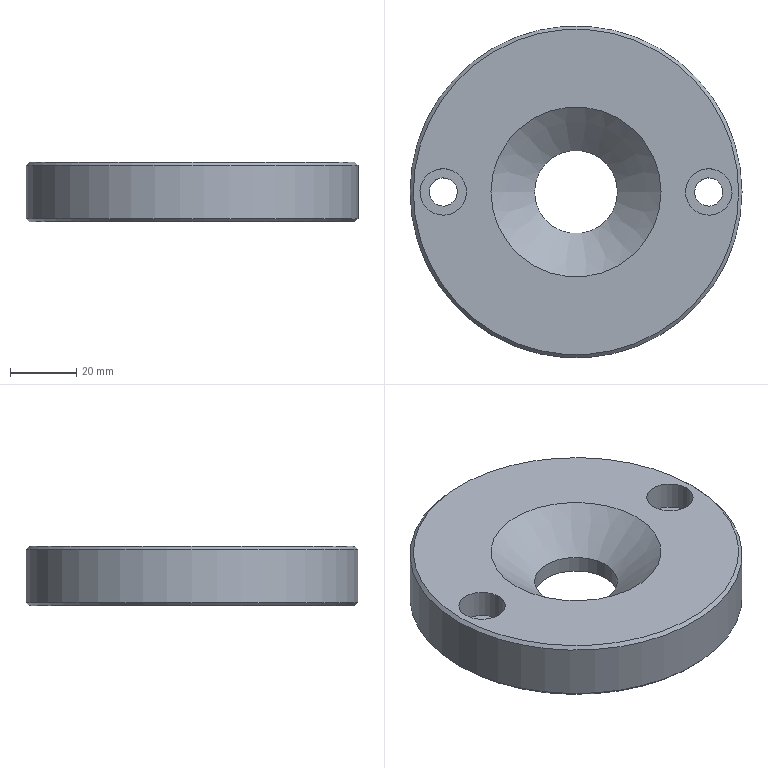Part | STEP file | P011002NF01-000 | 1 solid | 15 faces | box 100 x 100 x 18 mm | volume 119839 mm3 | cylinder 7 | plane 5 | cone 3 | commonest cylinder face diameters 8.5 x2 14 x2 25 x1 36 x1 100 x1
STEP:
#1=CARTESIAN_POINT('',(0.,0.,0.));
#2=DIRECTION('',(0.,0.,1.));
#3=DIRECTION('',(1.,0.,0.));
#4=AXIS2_PLACEMENT_3D('',#1,#2,#3);
#5=CARTESIAN_POINT('',(-12.5,0.,330.));
#6=VERTEX_POINT('',#5);
#7=CARTESIAN_POINT('',(12.5,0.,330.));
#8=VERTEX_POINT('',#7);
#9=CARTESIAN_POINT('',(0.,0.,330.));
#10=DIRECTION('',(0.,0.,1.));
#11=DIRECTION('',(-1.,0.,0.));
#12=AXIS2_PLACEMENT_3D('',#9,#10,#11);
#13=CIRCLE('',#12,12.5);
#14=CARTESIAN_POINT('',(0.,0.,330.));
#15=DIRECTION('',(0.,0.,-1.));
#16=DIRECTION('',(-0.9819,-0.1894,0.));
#17=AXIS2_PLACEMENT_3D('',#14,#15,#16);
#18=PLANE('',#17);
#19=CARTESIAN_POINT('',(12.274,2.368));
#20=CARTESIAN_POINT('',(16.375,-18.891));
#21=CARTESIAN_POINT('',(-4.086,-11.813));
#22=CARTESIAN_POINT('',(-24.547,-4.735));
#23=CARTESIAN_POINT('',(-8.187,9.446));
#24=CARTESIAN_POINT('',(8.173,23.626));
#25=CARTESIAN_POINT('',(12.274,2.368));
#26=(BOUNDED_CURVE()B_SPLINE_CURVE(2,(#19,#20,#21,#22,#23,#24,#25),.UNSPECIFIED.,.T.,.F.)B_SPLINE_CURVE_WITH_KNOTS((1,2,2,2,2,1),(-2.094,0.,2.094,4.189,6.283,8.378),.UNSPECIFIED.)CURVE()GEOMETRIC_REPRESENTATION_ITEM()RATIONAL_B_SPLINE_CURVE((1.,0.5,1.,0.5,1.,0.5,1.))REPRESENTATION_ITEM(''));
#27=(GEOMETRIC_REPRESENTATION_CONTEXT(2)PARAMETRIC_REPRESENTATION_CONTEXT()REPRESENTATION_CONTEXT('',''));
#28=DEFINITIONAL_REPRESENTATION('',(#26),#27);
#29=PCURVE('',#18,#28);
#30=CARTESIAN_POINT('',(0.,0.,289.));
#31=DIRECTION('',(0.,0.,1.));
#32=DIRECTION('',(0.9819,0.1894,0.));
#33=AXIS2_PLACEMENT_3D('',#30,#31,#32);
#34=CYLINDRICAL_SURFACE('',#33,12.5);
#35=CARTESIAN_POINT('',(9.234,41.));
#36=DIRECTION('',(1.,0.));
#37=VECTOR('',#36,1.);
#38=LINE('',#35,#37);
#39=(GEOMETRIC_REPRESENTATION_CONTEXT(2)PARAMETRIC_REPRESENTATION_CONTEXT()REPRESENTATION_CONTEXT('',''));
#40=DEFINITIONAL_REPRESENTATION('',(#38),#39);
#41=PCURVE('',#34,#40);
#42=SURFACE_CURVE('',#13,(#29,#41),.PCURVE_S1.);
#43=EDGE_CURVE('',#6,#8,#42,.T.);
#44=ORIENTED_EDGE('',*,*,#43,.T.);
#45=CARTESIAN_POINT('',(0.,0.,330.));
#46=DIRECTION('',(0.,0.,1.));
#47=DIRECTION('',(-1.,0.,0.));
#48=AXIS2_PLACEMENT_3D('',#45,#46,#47);
#49=CIRCLE('',#48,12.5);
#50=CARTESIAN_POINT('',(12.274,2.368));
#51=CARTESIAN_POINT('',(16.375,-18.891));
#52=CARTESIAN_POINT('',(-4.086,-11.813));
#53=CARTESIAN_POINT('',(-24.547,-4.735));
#54=CARTESIAN_POINT('',(-8.187,9.446));
#55=CARTESIAN_POINT('',(8.173,23.626));
#56=CARTESIAN_POINT('',(12.274,2.368));
#57=(BOUNDED_CURVE()B_SPLINE_CURVE(2,(#50,#51,#52,#53,#54,#55,#56),.UNSPECIFIED.,.T.,.F.)B_SPLINE_CURVE_WITH_KNOTS((1,2,2,2,2,1),(-2.094,0.,2.094,4.189,6.283,8.378),.UNSPECIFIED.)CURVE()GEOMETRIC_REPRESENTATION_ITEM()RATIONAL_B_SPLINE_CURVE((1.,0.5,1.,0.5,1.,0.5,1.))REPRESENTATION_ITEM(''));
#58=(GEOMETRIC_REPRESENTATION_CONTEXT(2)PARAMETRIC_REPRESENTATION_CONTEXT()REPRESENTATION_CONTEXT('',''));
#59=DEFINITIONAL_REPRESENTATION('',(#57),#58);
#60=PCURVE('',#18,#59);
#61=CARTESIAN_POINT('',(2.951,41.));
#62=DIRECTION('',(1.,0.));
#63=VECTOR('',#62,1.);
#64=LINE('',#61,#63);
#65=(GEOMETRIC_REPRESENTATION_CONTEXT(2)PARAMETRIC_REPRESENTATION_CONTEXT()REPRESENTATION_CONTEXT('',''));
#66=DEFINITIONAL_REPRESENTATION('',(#64),#65);
#67=PCURVE('',#34,#66);
#68=SURFACE_CURVE('',#49,(#60,#67),.PCURVE_S1.);
#69=EDGE_CURVE('',#8,#6,#68,.T.);
#70=ORIENTED_EDGE('',*,*,#69,.T.);
#71=EDGE_LOOP('',(#44,#70));
#72=FACE_BOUND('',#71,.T.);
#73=CARTESIAN_POINT('',(-18.,0.,330.));
#74=VERTEX_POINT('',#73);
#75=CARTESIAN_POINT('',(0.,0.,330.));
#76=DIRECTION('',(0.,0.,1.));
#77=DIRECTION('',(-1.,0.,0.));
#78=AXIS2_PLACEMENT_3D('',#75,#76,#77);
#79=CIRCLE('',#78,18.);
#80=CARTESIAN_POINT('',(17.674,3.409));
#81=CARTESIAN_POINT('',(23.58,-27.203));
#82=CARTESIAN_POINT('',(-5.884,-17.011));
#83=CARTESIAN_POINT('',(-35.348,-6.819));
#84=CARTESIAN_POINT('',(-11.79,13.602));
#85=CARTESIAN_POINT('',(11.769,34.022));
#86=CARTESIAN_POINT('',(17.674,3.409));
#87=(BOUNDED_CURVE()B_SPLINE_CURVE(2,(#80,#81,#82,#83,#84,#85,#86),.UNSPECIFIED.,.T.,.F.)B_SPLINE_CURVE_WITH_KNOTS((1,2,2,2,2,1),(-2.094,0.,2.094,4.189,6.283,8.378),.UNSPECIFIED.)CURVE()GEOMETRIC_REPRESENTATION_ITEM()RATIONAL_B_SPLINE_CURVE((1.,0.5,1.,0.5,1.,0.5,1.))REPRESENTATION_ITEM(''));
#88=(GEOMETRIC_REPRESENTATION_CONTEXT(2)PARAMETRIC_REPRESENTATION_CONTEXT()REPRESENTATION_CONTEXT('',''));
#89=DEFINITIONAL_REPRESENTATION('',(#87),#88);
#90=PCURVE('',#18,#89);
#91=CARTESIAN_POINT('',(0.,0.,289.));
#92=DIRECTION('',(0.,0.,1.));
#93=DIRECTION('',(0.9819,0.1894,0.));
#94=AXIS2_PLACEMENT_3D('',#91,#92,#93);
#95=CYLINDRICAL_SURFACE('',#94,18.);
#96=CARTESIAN_POINT('',(2.951,41.));
#97=DIRECTION('',(1.,0.));
#98=VECTOR('',#97,1.);
#99=LINE('',#96,#98);
#100=(GEOMETRIC_REPRESENTATION_CONTEXT(2)PARAMETRIC_REPRESENTATION_CONTEXT()REPRESENTATION_CONTEXT('',''));
#101=DEFINITIONAL_REPRESENTATION('',(#99),#100);
#102=PCURVE('',#95,#101);
#103=SURFACE_CURVE('',#79,(#90,#102),.PCURVE_S1.);
#104=EDGE_CURVE('',#74,#74,#103,.T.);
#105=ORIENTED_EDGE('',*,*,#104,.F.);
#106=EDGE_LOOP('',(#105));
#107=FACE_BOUND('',#106,.T.);
#108=ADVANCED_FACE('',(#72,#107),#18,.T.);
#109=CARTESIAN_POINT('',(-25.604,0.,346.));
#110=VERTEX_POINT('',#109);
#111=CARTESIAN_POINT('',(25.604,0.,346.));
#112=VERTEX_POINT('',#111);
#113=CARTESIAN_POINT('',(0.,0.,346.));
#114=DIRECTION('',(0.,0.,-1.));
#115=DIRECTION('',(-1.,0.,0.));
#116=AXIS2_PLACEMENT_3D('',#113,#114,#115);
#117=CIRCLE('',#116,25.604);
#118=CARTESIAN_POINT('',(0.,0.,335.004));
#119=DIRECTION('',(0.,0.,1.));
#120=DIRECTION('',(1.,0.,0.));
#121=AXIS2_PLACEMENT_3D('',#118,#119,#120);
#122=CONICAL_SURFACE('',#121,12.5,0.8727);
#123=CARTESIAN_POINT('',(3.142,10.996));
#124=DIRECTION('',(-1.,0.));
#125=VECTOR('',#124,1.);
#126=LINE('',#123,#125);
#127=(GEOMETRIC_REPRESENTATION_CONTEXT(2)PARAMETRIC_REPRESENTATION_CONTEXT()REPRESENTATION_CONTEXT('',''));
#128=DEFINITIONAL_REPRESENTATION('',(#126),#127);
#129=PCURVE('',#122,#128);
#130=CARTESIAN_POINT('',(331.581,-267.028,346.));
#131=DIRECTION('',(0.,0.,-1.));
#132=DIRECTION('',(-0.9819,-0.1894,0.));
#133=AXIS2_PLACEMENT_3D('',#130,#131,#132);
#134=PLANE('',#133);
#135=CARTESIAN_POINT('',(275.,325.));
#136=DIRECTION('',(0.9819,0.1894));
#137=AXIS2_PLACEMENT_2D('',#135,#136);
#138=CIRCLE('',#137,25.604);
#139=(GEOMETRIC_REPRESENTATION_CONTEXT(2)PARAMETRIC_REPRESENTATION_CONTEXT()REPRESENTATION_CONTEXT('',''));
#140=DEFINITIONAL_REPRESENTATION('',(#138),#139);
#141=PCURVE('',#134,#140);
#142=SURFACE_CURVE('',#117,(#129,#141),.PCURVE_S1.);
#143=EDGE_CURVE('',#110,#112,#142,.T.);
#144=ORIENTED_EDGE('',*,*,#143,.T.);
#145=CARTESIAN_POINT('',(12.5,0.,335.004));
#146=VERTEX_POINT('',#145);
#147=CARTESIAN_POINT('',(12.5,0.,335.004));
#148=CARTESIAN_POINT('',(25.604,0.,346.));
#149=B_SPLINE_CURVE_WITH_KNOTS('',1,(#147,#148),.UNSPECIFIED.,.F.,.F.,(2,2),(0.,17.106),.PIECEWISE_BEZIER_KNOTS.);
#150=CARTESIAN_POINT('',(0.,0.));
#151=DIRECTION('',(0.,1.));
#152=VECTOR('',#151,1.);
#153=LINE('',#150,#152);
#154=(GEOMETRIC_REPRESENTATION_CONTEXT(2)PARAMETRIC_REPRESENTATION_CONTEXT()REPRESENTATION_CONTEXT('',''));
#155=DEFINITIONAL_REPRESENTATION('',(#153),#154);
#156=PCURVE('',#122,#155);
#157=CARTESIAN_POINT('',(6.283,0.));
#158=DIRECTION('',(0.,1.));
#159=VECTOR('',#158,1.);
#160=LINE('',#157,#159);
#161=(GEOMETRIC_REPRESENTATION_CONTEXT(2)PARAMETRIC_REPRESENTATION_CONTEXT()REPRESENTATION_CONTEXT('',''));
#162=DEFINITIONAL_REPRESENTATION('',(#160),#161);
#163=PCURVE('',#122,#162);
#164=SEAM_CURVE('',#149,(#156,#163),.PCURVE_S1.);
#165=EDGE_CURVE('',#146,#112,#164,.T.);
#166=ORIENTED_EDGE('',*,*,#165,.F.);
#167=CARTESIAN_POINT('',(0.,0.,335.004));
#168=DIRECTION('',(0.,0.,1.));
#169=DIRECTION('',(1.,0.,0.));
#170=AXIS2_PLACEMENT_3D('',#167,#168,#169);
#171=CIRCLE('',#170,12.5);
#172=CARTESIAN_POINT('',(0.,0.));
#173=DIRECTION('',(1.,0.));
#174=VECTOR('',#173,1.);
#175=LINE('',#172,#174);
#176=(GEOMETRIC_REPRESENTATION_CONTEXT(2)PARAMETRIC_REPRESENTATION_CONTEXT()REPRESENTATION_CONTEXT('',''));
#177=DEFINITIONAL_REPRESENTATION('',(#175),#176);
#178=PCURVE('',#122,#177);
#179=CARTESIAN_POINT('',(6.093,46.004));
#180=DIRECTION('',(1.,0.));
#181=VECTOR('',#180,1.);
#182=LINE('',#179,#181);
#183=(GEOMETRIC_REPRESENTATION_CONTEXT(2)PARAMETRIC_REPRESENTATION_CONTEXT()REPRESENTATION_CONTEXT('',''));
#184=DEFINITIONAL_REPRESENTATION('',(#182),#183);
#185=PCURVE('',#34,#184);
#186=SURFACE_CURVE('',#171,(#178,#185),.PCURVE_S1.);
#187=EDGE_CURVE('',#146,#146,#186,.T.);
#188=ORIENTED_EDGE('',*,*,#187,.T.);
#189=ORIENTED_EDGE('',*,*,#165,.T.);
#190=CARTESIAN_POINT('',(0.,0.,346.));
#191=DIRECTION('',(0.,0.,-1.));
#192=DIRECTION('',(-1.,0.,0.));
#193=AXIS2_PLACEMENT_3D('',#190,#191,#192);
#194=CIRCLE('',#193,25.604);
#195=CARTESIAN_POINT('',(9.425,10.996));
#196=DIRECTION('',(-1.,0.));
#197=VECTOR('',#196,1.);
#198=LINE('',#195,#197);
#199=(GEOMETRIC_REPRESENTATION_CONTEXT(2)PARAMETRIC_REPRESENTATION_CONTEXT()REPRESENTATION_CONTEXT('',''));
#200=DEFINITIONAL_REPRESENTATION('',(#198),#199);
#201=PCURVE('',#122,#200);
#202=CARTESIAN_POINT('',(275.,325.));
#203=DIRECTION('',(0.9819,0.1894));
#204=AXIS2_PLACEMENT_2D('',#202,#203);
#205=CIRCLE('',#204,25.604);
#206=(GEOMETRIC_REPRESENTATION_CONTEXT(2)PARAMETRIC_REPRESENTATION_CONTEXT()REPRESENTATION_CONTEXT('',''));
#207=DEFINITIONAL_REPRESENTATION('',(#205),#206);
#208=PCURVE('',#134,#207);
#209=SURFACE_CURVE('',#194,(#201,#208),.PCURVE_S1.);
#210=EDGE_CURVE('',#112,#110,#209,.T.);
#211=ORIENTED_EDGE('',*,*,#210,.T.);
#212=EDGE_LOOP('',(#144,#166,#188,#189,#211));
#213=FACE_BOUND('',#212,.F.);
#214=ADVANCED_FACE('',(#213),#122,.F.);
#215=CARTESIAN_POINT('',(46.873,1.326,337.5));
#216=VERTEX_POINT('',#215);
#217=CARTESIAN_POINT('',(40.,0.,337.5));
#218=DIRECTION('',(0.,0.,1.));
#219=DIRECTION('',(0.9819,0.1894,0.));
#220=AXIS2_PLACEMENT_3D('',#217,#218,#219);
#221=CIRCLE('',#220,7.);
#222=CARTESIAN_POINT('',(0.,0.,337.5));
#223=DIRECTION('',(0.,0.,1.));
#224=DIRECTION('',(0.9819,0.1894,0.));
#225=AXIS2_PLACEMENT_3D('',#222,#223,#224);
#226=PLANE('',#225);
#227=CARTESIAN_POINT('',(39.276,-7.577));
#228=DIRECTION('',(1.,0.));
#229=AXIS2_PLACEMENT_2D('',#227,#228);
#230=CIRCLE('',#229,7.);
#231=(GEOMETRIC_REPRESENTATION_CONTEXT(2)PARAMETRIC_REPRESENTATION_CONTEXT()REPRESENTATION_CONTEXT('',''));
#232=DEFINITIONAL_REPRESENTATION('',(#230),#231);
#233=PCURVE('',#226,#232);
#234=CARTESIAN_POINT('',(40.,0.,282.));
#235=DIRECTION('',(0.,0.,1.));
#236=DIRECTION('',(0.9819,0.1894,0.));
#237=AXIS2_PLACEMENT_3D('',#234,#235,#236);
#238=CYLINDRICAL_SURFACE('',#237,7.);
#239=CARTESIAN_POINT('',(0.,55.5));
#240=DIRECTION('',(1.,0.));
#241=VECTOR('',#240,1.);
#242=LINE('',#239,#241);
#243=(GEOMETRIC_REPRESENTATION_CONTEXT(2)PARAMETRIC_REPRESENTATION_CONTEXT()REPRESENTATION_CONTEXT('',''));
#244=DEFINITIONAL_REPRESENTATION('',(#242),#243);
#245=PCURVE('',#238,#244);
#246=SURFACE_CURVE('',#221,(#233,#245),.PCURVE_S1.);
#247=EDGE_CURVE('',#216,#216,#246,.T.);
#248=ORIENTED_EDGE('',*,*,#247,.T.);
#249=EDGE_LOOP('',(#248));
#250=FACE_BOUND('',#249,.T.);
#251=CARTESIAN_POINT('',(44.173,0.805,337.5));
#252=VERTEX_POINT('',#251);
#253=CARTESIAN_POINT('',(40.,0.,337.5));
#254=DIRECTION('',(0.,0.,1.));
#255=DIRECTION('',(0.9819,0.1894,0.));
#256=AXIS2_PLACEMENT_3D('',#253,#254,#255);
#257=CIRCLE('',#256,4.25);
#258=CARTESIAN_POINT('',(39.276,-7.577));
#259=DIRECTION('',(1.,0.));
#260=AXIS2_PLACEMENT_2D('',#258,#259);
#261=CIRCLE('',#260,4.25);
#262=(GEOMETRIC_REPRESENTATION_CONTEXT(2)PARAMETRIC_REPRESENTATION_CONTEXT()REPRESENTATION_CONTEXT('',''));
#263=DEFINITIONAL_REPRESENTATION('',(#261),#262);
#264=PCURVE('',#226,#263);
#265=CARTESIAN_POINT('',(40.,0.,282.));
#266=DIRECTION('',(0.,0.,1.));
#267=DIRECTION('',(0.9819,0.1894,0.));
#268=AXIS2_PLACEMENT_3D('',#265,#266,#267);
#269=CYLINDRICAL_SURFACE('',#268,4.25);
#270=CARTESIAN_POINT('',(0.,55.5));
#271=DIRECTION('',(1.,0.));
#272=VECTOR('',#271,1.);
#273=LINE('',#270,#272);
#274=(GEOMETRIC_REPRESENTATION_CONTEXT(2)PARAMETRIC_REPRESENTATION_CONTEXT()REPRESENTATION_CONTEXT('',''));
#275=DEFINITIONAL_REPRESENTATION('',(#273),#274);
#276=PCURVE('',#269,#275);
#277=SURFACE_CURVE('',#257,(#264,#276),.PCURVE_S1.);
#278=EDGE_CURVE('',#252,#252,#277,.T.);
#279=ORIENTED_EDGE('',*,*,#278,.F.);
#280=EDGE_LOOP('',(#279));
#281=FACE_BOUND('',#280,.T.);
#282=ADVANCED_FACE('',(#250,#281),#226,.T.);
#283=ORIENTED_EDGE('',*,*,#143,.T.);
#284=ORIENTED_EDGE('',*,*,#210,.T.);
#285=EDGE_LOOP('',(#283,#284));
#286=FACE_BOUND('',#285,.T.);
#287=CARTESIAN_POINT('',(-49.,0.,346.));
#288=VERTEX_POINT('',#287);
#289=CARTESIAN_POINT('',(0.,0.,346.));
#290=DIRECTION('',(0.,0.,1.));
#291=DIRECTION('',(-1.,0.,0.));
#292=AXIS2_PLACEMENT_3D('',#289,#290,#291);
#293=CIRCLE('',#292,49.);
#294=CARTESIAN_POINT('',(323.113,334.281));
#295=CARTESIAN_POINT('',(339.189,250.947));
#296=CARTESIAN_POINT('',(258.981,278.692));
#297=CARTESIAN_POINT('',(178.774,306.437));
#298=CARTESIAN_POINT('',(242.906,362.026));
#299=CARTESIAN_POINT('',(307.037,417.615));
#300=CARTESIAN_POINT('',(323.113,334.281));
#301=(BOUNDED_CURVE()B_SPLINE_CURVE(2,(#294,#295,#296,#297,#298,#299,#300),.UNSPECIFIED.,.T.,.F.)B_SPLINE_CURVE_WITH_KNOTS((1,2,2,2,2,1),(-2.094,0.,2.094,4.189,6.283,8.378),.UNSPECIFIED.)CURVE()GEOMETRIC_REPRESENTATION_ITEM()RATIONAL_B_SPLINE_CURVE((1.,0.5,1.,0.5,1.,0.5,1.))REPRESENTATION_ITEM(''));
#302=(GEOMETRIC_REPRESENTATION_CONTEXT(2)PARAMETRIC_REPRESENTATION_CONTEXT()REPRESENTATION_CONTEXT('',''));
#303=DEFINITIONAL_REPRESENTATION('',(#301),#302);
#304=PCURVE('',#134,#303);
#305=CARTESIAN_POINT('',(0.,0.,346.));
#306=DIRECTION('',(0.,0.,-1.));
#307=DIRECTION('',(-1.,0.,0.));
#308=AXIS2_PLACEMENT_3D('',#305,#306,#307);
#309=CONICAL_SURFACE('',#308,49.,0.7854);
#310=CARTESIAN_POINT('',(6.283,0.));
#311=DIRECTION('',(-1.,0.));
#312=VECTOR('',#311,1.);
#313=LINE('',#310,#312);
#314=(GEOMETRIC_REPRESENTATION_CONTEXT(2)PARAMETRIC_REPRESENTATION_CONTEXT()REPRESENTATION_CONTEXT('',''));
#315=DEFINITIONAL_REPRESENTATION('',(#313),#314);
#316=PCURVE('',#309,#315);
#317=SURFACE_CURVE('',#293,(#304,#316),.PCURVE_S1.);
#318=EDGE_CURVE('',#288,#288,#317,.T.);
#319=ORIENTED_EDGE('',*,*,#318,.T.);
#320=EDGE_LOOP('',(#319));
#321=FACE_BOUND('',#320,.T.);
#322=CARTESIAN_POINT('',(-46.873,-1.326,346.));
#323=VERTEX_POINT('',#322);
#324=CARTESIAN_POINT('',(-33.127,1.326,346.));
#325=VERTEX_POINT('',#324);
#326=CARTESIAN_POINT('',(-40.,0.,346.));
#327=DIRECTION('',(0.,0.,1.));
#328=DIRECTION('',(-0.9819,-0.1894,0.));
#329=AXIS2_PLACEMENT_3D('',#326,#327,#328);
#330=CIRCLE('',#329,7.);
#331=CARTESIAN_POINT('',(321.276,332.577));
#332=CARTESIAN_POINT('',(321.276,320.452));
#333=CARTESIAN_POINT('',(310.776,326.514));
#334=CARTESIAN_POINT('',(300.276,332.577));
#335=CARTESIAN_POINT('',(310.776,338.639));
#336=CARTESIAN_POINT('',(321.276,344.701));
#337=CARTESIAN_POINT('',(321.276,332.577));
#338=(BOUNDED_CURVE()B_SPLINE_CURVE(2,(#331,#332,#333,#334,#335,#336,#337),.UNSPECIFIED.,.T.,.F.)B_SPLINE_CURVE_WITH_KNOTS((1,2,2,2,2,1),(-2.094,0.,2.094,4.189,6.283,8.378),.UNSPECIFIED.)CURVE()GEOMETRIC_REPRESENTATION_ITEM()RATIONAL_B_SPLINE_CURVE((1.,0.5,1.,0.5,1.,0.5,1.))REPRESENTATION_ITEM(''));
#339=(GEOMETRIC_REPRESENTATION_CONTEXT(2)PARAMETRIC_REPRESENTATION_CONTEXT()REPRESENTATION_CONTEXT('',''));
#340=DEFINITIONAL_REPRESENTATION('',(#338),#339);
#341=PCURVE('',#134,#340);
#342=CARTESIAN_POINT('',(-40.,0.,282.));
#343=DIRECTION('',(0.,0.,1.));
#344=DIRECTION('',(0.9819,0.1894,0.));
#345=AXIS2_PLACEMENT_3D('',#342,#343,#344);
#346=CYLINDRICAL_SURFACE('',#345,7.);
#347=CARTESIAN_POINT('',(3.142,64.));
#348=DIRECTION('',(1.,0.));
#349=VECTOR('',#348,1.);
#350=LINE('',#347,#349);
#351=(GEOMETRIC_REPRESENTATION_CONTEXT(2)PARAMETRIC_REPRESENTATION_CONTEXT()REPRESENTATION_CONTEXT('',''));
#352=DEFINITIONAL_REPRESENTATION('',(#350),#351);
#353=PCURVE('',#346,#352);
#354=SURFACE_CURVE('',#330,(#341,#353),.PCURVE_S1.);
#355=EDGE_CURVE('',#323,#325,#354,.T.);
#356=ORIENTED_EDGE('',*,*,#355,.F.);
#357=CARTESIAN_POINT('',(-40.,0.,346.));
#358=DIRECTION('',(0.,0.,1.));
#359=DIRECTION('',(-0.9819,-0.1894,0.));
#360=AXIS2_PLACEMENT_3D('',#357,#358,#359);
#361=CIRCLE('',#360,7.);
#362=CARTESIAN_POINT('',(321.276,332.577));
#363=CARTESIAN_POINT('',(321.276,320.452));
#364=CARTESIAN_POINT('',(310.776,326.514));
#365=CARTESIAN_POINT('',(300.276,332.577));
#366=CARTESIAN_POINT('',(310.776,338.639));
#367=CARTESIAN_POINT('',(321.276,344.701));
#368=CARTESIAN_POINT('',(321.276,332.577));
#369=(BOUNDED_CURVE()B_SPLINE_CURVE(2,(#362,#363,#364,#365,#366,#367,#368),.UNSPECIFIED.,.T.,.F.)B_SPLINE_CURVE_WITH_KNOTS((1,2,2,2,2,1),(-2.094,0.,2.094,4.189,6.283,8.378),.UNSPECIFIED.)CURVE()GEOMETRIC_REPRESENTATION_ITEM()RATIONAL_B_SPLINE_CURVE((1.,0.5,1.,0.5,1.,0.5,1.))REPRESENTATION_ITEM(''));
#370=(GEOMETRIC_REPRESENTATION_CONTEXT(2)PARAMETRIC_REPRESENTATION_CONTEXT()REPRESENTATION_CONTEXT('',''));
#371=DEFINITIONAL_REPRESENTATION('',(#369),#370);
#372=PCURVE('',#134,#371);
#373=CARTESIAN_POINT('',(-3.142,64.));
#374=DIRECTION('',(1.,0.));
#375=VECTOR('',#374,1.);
#376=LINE('',#373,#375);
#377=(GEOMETRIC_REPRESENTATION_CONTEXT(2)PARAMETRIC_REPRESENTATION_CONTEXT()REPRESENTATION_CONTEXT('',''));
#378=DEFINITIONAL_REPRESENTATION('',(#376),#377);
#379=PCURVE('',#346,#378);
#380=SURFACE_CURVE('',#361,(#372,#379),.PCURVE_S1.);
#381=EDGE_CURVE('',#325,#323,#380,.T.);
#382=ORIENTED_EDGE('',*,*,#381,.F.);
#383=EDGE_LOOP('',(#356,#382));
#384=FACE_BOUND('',#383,.T.);
#385=CARTESIAN_POINT('',(33.127,-1.326,346.));
#386=VERTEX_POINT('',#385);
#387=CARTESIAN_POINT('',(46.873,1.326,346.));
#388=VERTEX_POINT('',#387);
#389=CARTESIAN_POINT('',(40.,0.,346.));
#390=DIRECTION('',(0.,0.,-1.));
#391=DIRECTION('',(-0.9819,-0.1894,0.));
#392=AXIS2_PLACEMENT_3D('',#389,#390,#391);
#393=CIRCLE('',#392,7.);
#394=CARTESIAN_POINT('',(235.724,317.423));
#395=DIRECTION('',(1.,0.));
#396=AXIS2_PLACEMENT_2D('',#394,#395);
#397=CIRCLE('',#396,7.);
#398=(GEOMETRIC_REPRESENTATION_CONTEXT(2)PARAMETRIC_REPRESENTATION_CONTEXT()REPRESENTATION_CONTEXT('',''));
#399=DEFINITIONAL_REPRESENTATION('',(#397),#398);
#400=PCURVE('',#134,#399);
#401=CARTESIAN_POINT('',(3.142,64.));
#402=DIRECTION('',(-1.,0.));
#403=VECTOR('',#402,1.);
#404=LINE('',#401,#403);
#405=(GEOMETRIC_REPRESENTATION_CONTEXT(2)PARAMETRIC_REPRESENTATION_CONTEXT()REPRESENTATION_CONTEXT('',''));
#406=DEFINITIONAL_REPRESENTATION('',(#404),#405);
#407=PCURVE('',#238,#406);
#408=SURFACE_CURVE('',#393,(#400,#407),.PCURVE_S1.);
#409=EDGE_CURVE('',#386,#388,#408,.T.);
#410=ORIENTED_EDGE('',*,*,#409,.T.);
#411=CARTESIAN_POINT('',(40.,0.,346.));
#412=DIRECTION('',(0.,0.,-1.));
#413=DIRECTION('',(-0.9819,-0.1894,0.));
#414=AXIS2_PLACEMENT_3D('',#411,#412,#413);
#415=CIRCLE('',#414,7.);
#416=CARTESIAN_POINT('',(235.724,317.423));
#417=DIRECTION('',(1.,0.));
#418=AXIS2_PLACEMENT_2D('',#416,#417);
#419=CIRCLE('',#418,7.);
#420=(GEOMETRIC_REPRESENTATION_CONTEXT(2)PARAMETRIC_REPRESENTATION_CONTEXT()REPRESENTATION_CONTEXT('',''));
#421=DEFINITIONAL_REPRESENTATION('',(#419),#420);
#422=PCURVE('',#134,#421);
#423=CARTESIAN_POINT('',(9.425,64.));
#424=DIRECTION('',(-1.,0.));
#425=VECTOR('',#424,1.);
#426=LINE('',#423,#425);
#427=(GEOMETRIC_REPRESENTATION_CONTEXT(2)PARAMETRIC_REPRESENTATION_CONTEXT()REPRESENTATION_CONTEXT('',''));
#428=DEFINITIONAL_REPRESENTATION('',(#426),#427);
#429=PCURVE('',#238,#428);
#430=SURFACE_CURVE('',#415,(#422,#429),.PCURVE_S1.);
#431=EDGE_CURVE('',#388,#386,#430,.T.);
#432=ORIENTED_EDGE('',*,*,#431,.T.);
#433=EDGE_LOOP('',(#410,#432));
#434=FACE_BOUND('',#433,.T.);
#435=ADVANCED_FACE('',(#286,#321,#384,#434),#134,.F.);
#436=CARTESIAN_POINT('',(-50.,0.,345.));
#437=VERTEX_POINT('',#436);
#438=CARTESIAN_POINT('',(0.,0.,345.));
#439=DIRECTION('',(0.,0.,-1.));
#440=DIRECTION('',(-1.,0.,0.));
#441=AXIS2_PLACEMENT_3D('',#438,#439,#440);
#442=CIRCLE('',#441,50.);
#443=CARTESIAN_POINT('',(0.,0.,289.));
#444=DIRECTION('',(0.,0.,1.));
#445=DIRECTION('',(0.9819,0.1894,0.));
#446=AXIS2_PLACEMENT_3D('',#443,#444,#445);
#447=CYLINDRICAL_SURFACE('',#446,50.);
#448=CARTESIAN_POINT('',(9.234,56.));
#449=DIRECTION('',(-1.,0.));
#450=VECTOR('',#449,1.);
#451=LINE('',#448,#450);
#452=(GEOMETRIC_REPRESENTATION_CONTEXT(2)PARAMETRIC_REPRESENTATION_CONTEXT()REPRESENTATION_CONTEXT('',''));
#453=DEFINITIONAL_REPRESENTATION('',(#451),#452);
#454=PCURVE('',#447,#453);
#455=CARTESIAN_POINT('',(0.,1.));
#456=DIRECTION('',(1.,0.));
#457=VECTOR('',#456,1.);
#458=LINE('',#455,#457);
#459=(GEOMETRIC_REPRESENTATION_CONTEXT(2)PARAMETRIC_REPRESENTATION_CONTEXT()REPRESENTATION_CONTEXT('',''));
#460=DEFINITIONAL_REPRESENTATION('',(#458),#459);
#461=PCURVE('',#309,#460);
#462=SURFACE_CURVE('',#442,(#454,#461),.PCURVE_S1.);
#463=EDGE_CURVE('',#437,#437,#462,.T.);
#464=ORIENTED_EDGE('',*,*,#463,.T.);
#465=CARTESIAN_POINT('',(-50.,0.,329.));
#466=VERTEX_POINT('',#465);
#467=CARTESIAN_POINT('',(-50.,0.,329.));
#468=CARTESIAN_POINT('',(-50.,0.,345.));
#469=B_SPLINE_CURVE_WITH_KNOTS('',1,(#467,#468),.UNSPECIFIED.,.F.,.F.,(2,2),(40.,56.),.PIECEWISE_BEZIER_KNOTS.);
#470=CARTESIAN_POINT('',(2.951,0.));
#471=DIRECTION('',(0.,1.));
#472=VECTOR('',#471,1.);
#473=LINE('',#470,#472);
#474=(GEOMETRIC_REPRESENTATION_CONTEXT(2)PARAMETRIC_REPRESENTATION_CONTEXT()REPRESENTATION_CONTEXT('',''));
#475=DEFINITIONAL_REPRESENTATION('',(#473),#474);
#476=PCURVE('',#447,#475);
#477=CARTESIAN_POINT('',(9.234,0.));
#478=DIRECTION('',(0.,1.));
#479=VECTOR('',#478,1.);
#480=LINE('',#477,#479);
#481=(GEOMETRIC_REPRESENTATION_CONTEXT(2)PARAMETRIC_REPRESENTATION_CONTEXT()REPRESENTATION_CONTEXT('',''));
#482=DEFINITIONAL_REPRESENTATION('',(#480),#481);
#483=PCURVE('',#447,#482);
#484=SEAM_CURVE('',#469,(#476,#483),.PCURVE_S1.);
#485=EDGE_CURVE('',#466,#437,#484,.T.);
#486=ORIENTED_EDGE('',*,*,#485,.F.);
#487=CARTESIAN_POINT('',(0.,0.,329.));
#488=DIRECTION('',(0.,0.,1.));
#489=DIRECTION('',(-1.,0.,0.));
#490=AXIS2_PLACEMENT_3D('',#487,#488,#489);
#491=CIRCLE('',#490,50.);
#492=CARTESIAN_POINT('',(2.951,40.));
#493=DIRECTION('',(1.,0.));
#494=VECTOR('',#493,1.);
#495=LINE('',#492,#494);
#496=(GEOMETRIC_REPRESENTATION_CONTEXT(2)PARAMETRIC_REPRESENTATION_CONTEXT()REPRESENTATION_CONTEXT('',''));
#497=DEFINITIONAL_REPRESENTATION('',(#495),#496);
#498=PCURVE('',#447,#497);
#499=CARTESIAN_POINT('',(0.,0.,329.));
#500=DIRECTION('',(0.,0.,1.));
#501=DIRECTION('',(1.,0.,0.));
#502=AXIS2_PLACEMENT_3D('',#499,#500,#501);
#503=CONICAL_SURFACE('',#502,50.,0.7854);
#504=CARTESIAN_POINT('',(3.142,0.));
#505=DIRECTION('',(1.,0.));
#506=VECTOR('',#505,1.);
#507=LINE('',#504,#506);
#508=(GEOMETRIC_REPRESENTATION_CONTEXT(2)PARAMETRIC_REPRESENTATION_CONTEXT()REPRESENTATION_CONTEXT('',''));
#509=DEFINITIONAL_REPRESENTATION('',(#507),#508);
#510=PCURVE('',#503,#509);
#511=SURFACE_CURVE('',#491,(#498,#510),.PCURVE_S1.);
#512=EDGE_CURVE('',#466,#466,#511,.T.);
#513=ORIENTED_EDGE('',*,*,#512,.T.);
#514=ORIENTED_EDGE('',*,*,#485,.T.);
#515=EDGE_LOOP('',(#464,#486,#513,#514));
#516=FACE_BOUND('',#515,.T.);
#517=ADVANCED_FACE('',(#516),#447,.T.);
#518=ORIENTED_EDGE('',*,*,#43,.T.);
#519=CARTESIAN_POINT('',(12.5,0.,330.));
#520=CARTESIAN_POINT('',(12.5,0.,335.004));
#521=B_SPLINE_CURVE_WITH_KNOTS('',1,(#519,#520),.UNSPECIFIED.,.F.,.F.,(2,2),(41.,46.004),.PIECEWISE_BEZIER_KNOTS.);
#522=CARTESIAN_POINT('',(12.376,0.));
#523=DIRECTION('',(0.,1.));
#524=VECTOR('',#523,1.);
#525=LINE('',#522,#524);
#526=(GEOMETRIC_REPRESENTATION_CONTEXT(2)PARAMETRIC_REPRESENTATION_CONTEXT()REPRESENTATION_CONTEXT('',''));
#527=DEFINITIONAL_REPRESENTATION('',(#525),#526);
#528=PCURVE('',#34,#527);
#529=CARTESIAN_POINT('',(6.093,0.));
#530=DIRECTION('',(0.,1.));
#531=VECTOR('',#530,1.);
#532=LINE('',#529,#531);
#533=(GEOMETRIC_REPRESENTATION_CONTEXT(2)PARAMETRIC_REPRESENTATION_CONTEXT()REPRESENTATION_CONTEXT('',''));
#534=DEFINITIONAL_REPRESENTATION('',(#532),#533);
#535=PCURVE('',#34,#534);
#536=SEAM_CURVE('',#521,(#528,#535),.PCURVE_S1.);
#537=EDGE_CURVE('',#8,#146,#536,.T.);
#538=ORIENTED_EDGE('',*,*,#537,.T.);
#539=ORIENTED_EDGE('',*,*,#187,.F.);
#540=ORIENTED_EDGE('',*,*,#537,.F.);
#541=ORIENTED_EDGE('',*,*,#69,.T.);
#542=EDGE_LOOP('',(#518,#538,#539,#540,#541));
#543=FACE_BOUND('',#542,.F.);
#544=ADVANCED_FACE('',(#543),#34,.F.);
#545=CARTESIAN_POINT('',(-35.827,0.805,337.5));
#546=VERTEX_POINT('',#545);
#547=CARTESIAN_POINT('',(-40.,0.,337.5));
#548=DIRECTION('',(0.,0.,-1.));
#549=DIRECTION('',(0.9819,0.1894,0.));
#550=AXIS2_PLACEMENT_3D('',#547,#548,#549);
#551=CIRCLE('',#550,4.25);
#552=CARTESIAN_POINT('',(0.,0.,337.5));
#553=DIRECTION('',(0.,0.,1.));
#554=DIRECTION('',(0.9819,0.1894,0.));
#555=AXIS2_PLACEMENT_3D('',#552,#553,#554);
#556=PLANE('',#555);
#557=CARTESIAN_POINT('',(-35.026,7.577));
#558=CARTESIAN_POINT('',(-35.026,0.2154));
#559=CARTESIAN_POINT('',(-41.401,3.896));
#560=CARTESIAN_POINT('',(-47.776,7.577));
#561=CARTESIAN_POINT('',(-41.401,11.257));
#562=CARTESIAN_POINT('',(-35.026,14.938));
#563=CARTESIAN_POINT('',(-35.026,7.577));
#564=(BOUNDED_CURVE()B_SPLINE_CURVE(2,(#557,#558,#559,#560,#561,#562,#563),.UNSPECIFIED.,.T.,.F.)B_SPLINE_CURVE_WITH_KNOTS((1,2,2,2,2,1),(-2.094,0.,2.094,4.189,6.283,8.378),.UNSPECIFIED.)CURVE()GEOMETRIC_REPRESENTATION_ITEM()RATIONAL_B_SPLINE_CURVE((1.,0.5,1.,0.5,1.,0.5,1.))REPRESENTATION_ITEM(''));
#565=(GEOMETRIC_REPRESENTATION_CONTEXT(2)PARAMETRIC_REPRESENTATION_CONTEXT()REPRESENTATION_CONTEXT('',''));
#566=DEFINITIONAL_REPRESENTATION('',(#564),#565);
#567=PCURVE('',#556,#566);
#568=CARTESIAN_POINT('',(-40.,0.,282.));
#569=DIRECTION('',(0.,0.,1.));
#570=DIRECTION('',(0.9819,0.1894,0.));
#571=AXIS2_PLACEMENT_3D('',#568,#569,#570);
#572=CYLINDRICAL_SURFACE('',#571,4.25);
#573=CARTESIAN_POINT('',(6.283,55.5));
#574=DIRECTION('',(-1.,0.));
#575=VECTOR('',#574,1.);
#576=LINE('',#573,#575);
#577=(GEOMETRIC_REPRESENTATION_CONTEXT(2)PARAMETRIC_REPRESENTATION_CONTEXT()REPRESENTATION_CONTEXT('',''));
#578=DEFINITIONAL_REPRESENTATION('',(#576),#577);
#579=PCURVE('',#572,#578);
#580=SURFACE_CURVE('',#551,(#567,#579),.PCURVE_S1.);
#581=EDGE_CURVE('',#546,#546,#580,.T.);
#582=ORIENTED_EDGE('',*,*,#581,.T.);
#583=EDGE_LOOP('',(#582));
#584=FACE_BOUND('',#583,.T.);
#585=CARTESIAN_POINT('',(-33.127,1.326,337.5));
#586=VERTEX_POINT('',#585);
#587=CARTESIAN_POINT('',(-40.,0.,337.5));
#588=DIRECTION('',(0.,0.,-1.));
#589=DIRECTION('',(0.9819,0.1894,0.));
#590=AXIS2_PLACEMENT_3D('',#587,#588,#589);
#591=CIRCLE('',#590,7.);
#592=CARTESIAN_POINT('',(-32.276,7.577));
#593=CARTESIAN_POINT('',(-32.276,-4.548));
#594=CARTESIAN_POINT('',(-42.776,1.514));
#595=CARTESIAN_POINT('',(-53.276,7.577));
#596=CARTESIAN_POINT('',(-42.776,13.639));
#597=CARTESIAN_POINT('',(-32.276,19.701));
#598=CARTESIAN_POINT('',(-32.276,7.577));
#599=(BOUNDED_CURVE()B_SPLINE_CURVE(2,(#592,#593,#594,#595,#596,#597,#598),.UNSPECIFIED.,.T.,.F.)B_SPLINE_CURVE_WITH_KNOTS((1,2,2,2,2,1),(-2.094,0.,2.094,4.189,6.283,8.378),.UNSPECIFIED.)CURVE()GEOMETRIC_REPRESENTATION_ITEM()RATIONAL_B_SPLINE_CURVE((1.,0.5,1.,0.5,1.,0.5,1.))REPRESENTATION_ITEM(''));
#600=(GEOMETRIC_REPRESENTATION_CONTEXT(2)PARAMETRIC_REPRESENTATION_CONTEXT()REPRESENTATION_CONTEXT('',''));
#601=DEFINITIONAL_REPRESENTATION('',(#599),#600);
#602=PCURVE('',#556,#601);
#603=CARTESIAN_POINT('',(6.283,55.5));
#604=DIRECTION('',(-1.,0.));
#605=VECTOR('',#604,1.);
#606=LINE('',#603,#605);
#607=(GEOMETRIC_REPRESENTATION_CONTEXT(2)PARAMETRIC_REPRESENTATION_CONTEXT()REPRESENTATION_CONTEXT('',''));
#608=DEFINITIONAL_REPRESENTATION('',(#606),#607);
#609=PCURVE('',#346,#608);
#610=SURFACE_CURVE('',#591,(#602,#609),.PCURVE_S1.);
#611=EDGE_CURVE('',#586,#586,#610,.T.);
#612=ORIENTED_EDGE('',*,*,#611,.F.);
#613=EDGE_LOOP('',(#612));
#614=FACE_BOUND('',#613,.T.);
#615=ADVANCED_FACE('',(#584,#614),#556,.T.);
#616=ORIENTED_EDGE('',*,*,#611,.F.);
#617=CARTESIAN_POINT('',(-33.127,1.326,337.5));
#618=CARTESIAN_POINT('',(-33.127,1.326,346.));
#619=B_SPLINE_CURVE_WITH_KNOTS('',1,(#617,#618),.UNSPECIFIED.,.F.,.F.,(2,2),(55.5,64.),.PIECEWISE_BEZIER_KNOTS.);
#620=CARTESIAN_POINT('',(6.283,0.));
#621=DIRECTION('',(0.,1.));
#622=VECTOR('',#621,1.);
#623=LINE('',#620,#622);
#624=(GEOMETRIC_REPRESENTATION_CONTEXT(2)PARAMETRIC_REPRESENTATION_CONTEXT()REPRESENTATION_CONTEXT('',''));
#625=DEFINITIONAL_REPRESENTATION('',(#623),#624);
#626=PCURVE('',#346,#625);
#627=CARTESIAN_POINT('',(0.,0.));
#628=DIRECTION('',(0.,1.));
#629=VECTOR('',#628,1.);
#630=LINE('',#627,#629);
#631=(GEOMETRIC_REPRESENTATION_CONTEXT(2)PARAMETRIC_REPRESENTATION_CONTEXT()REPRESENTATION_CONTEXT('',''));
#632=DEFINITIONAL_REPRESENTATION('',(#630),#631);
#633=PCURVE('',#346,#632);
#634=SEAM_CURVE('',#619,(#626,#633),.PCURVE_S1.);
#635=EDGE_CURVE('',#586,#325,#634,.T.);
#636=ORIENTED_EDGE('',*,*,#635,.T.);
#637=ORIENTED_EDGE('',*,*,#355,.F.);
#638=ORIENTED_EDGE('',*,*,#381,.F.);
#639=ORIENTED_EDGE('',*,*,#635,.F.);
#640=EDGE_LOOP('',(#616,#636,#637,#638,#639));
#641=FACE_BOUND('',#640,.F.);
#642=ADVANCED_FACE('',(#641),#346,.F.);
#643=ORIENTED_EDGE('',*,*,#247,.T.);
#644=CARTESIAN_POINT('',(46.873,1.326,337.5));
#645=CARTESIAN_POINT('',(46.873,1.326,346.));
#646=B_SPLINE_CURVE_WITH_KNOTS('',1,(#644,#645),.UNSPECIFIED.,.F.,.F.,(2,2),(55.5,64.),.PIECEWISE_BEZIER_KNOTS.);
#647=CARTESIAN_POINT('',(6.283,0.));
#648=DIRECTION('',(0.,1.));
#649=VECTOR('',#648,1.);
#650=LINE('',#647,#649);
#651=(GEOMETRIC_REPRESENTATION_CONTEXT(2)PARAMETRIC_REPRESENTATION_CONTEXT()REPRESENTATION_CONTEXT('',''));
#652=DEFINITIONAL_REPRESENTATION('',(#650),#651);
#653=PCURVE('',#238,#652);
#654=CARTESIAN_POINT('',(0.,0.));
#655=DIRECTION('',(0.,1.));
#656=VECTOR('',#655,1.);
#657=LINE('',#654,#656);
#658=(GEOMETRIC_REPRESENTATION_CONTEXT(2)PARAMETRIC_REPRESENTATION_CONTEXT()REPRESENTATION_CONTEXT('',''));
#659=DEFINITIONAL_REPRESENTATION('',(#657),#658);
#660=PCURVE('',#238,#659);
#661=SEAM_CURVE('',#646,(#653,#660),.PCURVE_S1.);
#662=EDGE_CURVE('',#216,#388,#661,.T.);
#663=ORIENTED_EDGE('',*,*,#662,.T.);
#664=ORIENTED_EDGE('',*,*,#431,.T.);
#665=ORIENTED_EDGE('',*,*,#409,.T.);
#666=ORIENTED_EDGE('',*,*,#662,.F.);
#667=EDGE_LOOP('',(#643,#663,#664,#665,#666));
#668=FACE_BOUND('',#667,.F.);
#669=ADVANCED_FACE('',(#668),#238,.F.);
#670=ORIENTED_EDGE('',*,*,#278,.F.);
#671=CARTESIAN_POINT('',(44.173,0.805,328.));
#672=VERTEX_POINT('',#671);
#673=CARTESIAN_POINT('',(44.173,0.805,328.));
#674=CARTESIAN_POINT('',(44.173,0.805,337.5));
#675=B_SPLINE_CURVE_WITH_KNOTS('',1,(#673,#674),.UNSPECIFIED.,.F.,.F.,(2,2),(46.,55.5),.PIECEWISE_BEZIER_KNOTS.);
#676=CARTESIAN_POINT('',(0.,0.));
#677=DIRECTION('',(0.,1.));
#678=VECTOR('',#677,1.);
#679=LINE('',#676,#678);
#680=(GEOMETRIC_REPRESENTATION_CONTEXT(2)PARAMETRIC_REPRESENTATION_CONTEXT()REPRESENTATION_CONTEXT('',''));
#681=DEFINITIONAL_REPRESENTATION('',(#679),#680);
#682=PCURVE('',#269,#681);
#683=CARTESIAN_POINT('',(6.283,0.));
#684=DIRECTION('',(0.,1.));
#685=VECTOR('',#684,1.);
#686=LINE('',#683,#685);
#687=(GEOMETRIC_REPRESENTATION_CONTEXT(2)PARAMETRIC_REPRESENTATION_CONTEXT()REPRESENTATION_CONTEXT('',''));
#688=DEFINITIONAL_REPRESENTATION('',(#686),#687);
#689=PCURVE('',#269,#688);
#690=SEAM_CURVE('',#675,(#682,#689),.PCURVE_S1.);
#691=EDGE_CURVE('',#672,#252,#690,.T.);
#692=ORIENTED_EDGE('',*,*,#691,.F.);
#693=CARTESIAN_POINT('',(35.827,-0.805,328.));
#694=VERTEX_POINT('',#693);
#695=CARTESIAN_POINT('',(40.,0.,328.));
#696=DIRECTION('',(0.,0.,1.));
#697=DIRECTION('',(-0.9819,-0.1894,0.));
#698=AXIS2_PLACEMENT_3D('',#695,#696,#697);
#699=CIRCLE('',#698,4.25);
#700=CARTESIAN_POINT('',(-3.142,46.));
#701=DIRECTION('',(1.,0.));
#702=VECTOR('',#701,1.);
#703=LINE('',#700,#702);
#704=(GEOMETRIC_REPRESENTATION_CONTEXT(2)PARAMETRIC_REPRESENTATION_CONTEXT()REPRESENTATION_CONTEXT('',''));
#705=DEFINITIONAL_REPRESENTATION('',(#703),#704);
#706=PCURVE('',#269,#705);
#707=CARTESIAN_POINT('',(0.,0.,328.));
#708=DIRECTION('',(0.,0.,-1.));
#709=DIRECTION('',(-0.9819,-0.1894,0.));
#710=AXIS2_PLACEMENT_3D('',#707,#708,#709);
#711=PLANE('',#710);
#712=CARTESIAN_POINT('',(-35.026,-7.577));
#713=CARTESIAN_POINT('',(-35.026,-14.938));
#714=CARTESIAN_POINT('',(-41.401,-11.257));
#715=CARTESIAN_POINT('',(-47.776,-7.577));
#716=CARTESIAN_POINT('',(-41.401,-3.896));
#717=CARTESIAN_POINT('',(-35.026,-0.2154));
#718=CARTESIAN_POINT('',(-35.026,-7.577));
#719=(BOUNDED_CURVE()B_SPLINE_CURVE(2,(#712,#713,#714,#715,#716,#717,#718),.UNSPECIFIED.,.T.,.F.)B_SPLINE_CURVE_WITH_KNOTS((1,2,2,2,2,1),(-2.094,0.,2.094,4.189,6.283,8.378),.UNSPECIFIED.)CURVE()GEOMETRIC_REPRESENTATION_ITEM()RATIONAL_B_SPLINE_CURVE((1.,0.5,1.,0.5,1.,0.5,1.))REPRESENTATION_ITEM(''));
#720=(GEOMETRIC_REPRESENTATION_CONTEXT(2)PARAMETRIC_REPRESENTATION_CONTEXT()REPRESENTATION_CONTEXT('',''));
#721=DEFINITIONAL_REPRESENTATION('',(#719),#720);
#722=PCURVE('',#711,#721);
#723=SURFACE_CURVE('',#699,(#706,#722),.PCURVE_S1.);
#724=EDGE_CURVE('',#672,#694,#723,.T.);
#725=ORIENTED_EDGE('',*,*,#724,.T.);
#726=CARTESIAN_POINT('',(40.,0.,328.));
#727=DIRECTION('',(0.,0.,1.));
#728=DIRECTION('',(-0.9819,-0.1894,0.));
#729=AXIS2_PLACEMENT_3D('',#726,#727,#728);
#730=CIRCLE('',#729,4.25);
#731=CARTESIAN_POINT('',(3.142,46.));
#732=DIRECTION('',(1.,0.));
#733=VECTOR('',#732,1.);
#734=LINE('',#731,#733);
#735=(GEOMETRIC_REPRESENTATION_CONTEXT(2)PARAMETRIC_REPRESENTATION_CONTEXT()REPRESENTATION_CONTEXT('',''));
#736=DEFINITIONAL_REPRESENTATION('',(#734),#735);
#737=PCURVE('',#269,#736);
#738=CARTESIAN_POINT('',(-35.026,-7.577));
#739=CARTESIAN_POINT('',(-35.026,-14.938));
#740=CARTESIAN_POINT('',(-41.401,-11.257));
#741=CARTESIAN_POINT('',(-47.776,-7.577));
#742=CARTESIAN_POINT('',(-41.401,-3.896));
#743=CARTESIAN_POINT('',(-35.026,-0.2154));
#744=CARTESIAN_POINT('',(-35.026,-7.577));
#745=(BOUNDED_CURVE()B_SPLINE_CURVE(2,(#738,#739,#740,#741,#742,#743,#744),.UNSPECIFIED.,.T.,.F.)B_SPLINE_CURVE_WITH_KNOTS((1,2,2,2,2,1),(-2.094,0.,2.094,4.189,6.283,8.378),.UNSPECIFIED.)CURVE()GEOMETRIC_REPRESENTATION_ITEM()RATIONAL_B_SPLINE_CURVE((1.,0.5,1.,0.5,1.,0.5,1.))REPRESENTATION_ITEM(''));
#746=(GEOMETRIC_REPRESENTATION_CONTEXT(2)PARAMETRIC_REPRESENTATION_CONTEXT()REPRESENTATION_CONTEXT('',''));
#747=DEFINITIONAL_REPRESENTATION('',(#745),#746);
#748=PCURVE('',#711,#747);
#749=SURFACE_CURVE('',#730,(#737,#748),.PCURVE_S1.);
#750=EDGE_CURVE('',#694,#672,#749,.T.);
#751=ORIENTED_EDGE('',*,*,#750,.T.);
#752=ORIENTED_EDGE('',*,*,#691,.T.);
#753=EDGE_LOOP('',(#670,#692,#725,#751,#752));
#754=FACE_BOUND('',#753,.F.);
#755=ADVANCED_FACE('',(#754),#269,.F.);
#756=ORIENTED_EDGE('',*,*,#581,.T.);
#757=CARTESIAN_POINT('',(-35.827,0.805,328.));
#758=VERTEX_POINT('',#757);
#759=CARTESIAN_POINT('',(-35.827,0.805,328.));
#760=CARTESIAN_POINT('',(-35.827,0.805,337.5));
#761=B_SPLINE_CURVE_WITH_KNOTS('',1,(#759,#760),.UNSPECIFIED.,.F.,.F.,(2,2),(46.,55.5),.PIECEWISE_BEZIER_KNOTS.);
#762=CARTESIAN_POINT('',(0.,0.));
#763=DIRECTION('',(0.,1.));
#764=VECTOR('',#763,1.);
#765=LINE('',#762,#764);
#766=(GEOMETRIC_REPRESENTATION_CONTEXT(2)PARAMETRIC_REPRESENTATION_CONTEXT()REPRESENTATION_CONTEXT('',''));
#767=DEFINITIONAL_REPRESENTATION('',(#765),#766);
#768=PCURVE('',#572,#767);
#769=CARTESIAN_POINT('',(6.283,0.));
#770=DIRECTION('',(0.,1.));
#771=VECTOR('',#770,1.);
#772=LINE('',#769,#771);
#773=(GEOMETRIC_REPRESENTATION_CONTEXT(2)PARAMETRIC_REPRESENTATION_CONTEXT()REPRESENTATION_CONTEXT('',''));
#774=DEFINITIONAL_REPRESENTATION('',(#772),#773);
#775=PCURVE('',#572,#774);
#776=SEAM_CURVE('',#761,(#768,#775),.PCURVE_S1.);
#777=EDGE_CURVE('',#758,#546,#776,.T.);
#778=ORIENTED_EDGE('',*,*,#777,.F.);
#779=CARTESIAN_POINT('',(-44.173,-0.805,328.));
#780=VERTEX_POINT('',#779);
#781=CARTESIAN_POINT('',(-40.,0.,328.));
#782=DIRECTION('',(0.,0.,-1.));
#783=DIRECTION('',(-0.9819,-0.1894,0.));
#784=AXIS2_PLACEMENT_3D('',#781,#782,#783);
#785=CIRCLE('',#784,4.25);
#786=CARTESIAN_POINT('',(3.142,46.));
#787=DIRECTION('',(-1.,0.));
#788=VECTOR('',#787,1.);
#789=LINE('',#786,#788);
#790=(GEOMETRIC_REPRESENTATION_CONTEXT(2)PARAMETRIC_REPRESENTATION_CONTEXT()REPRESENTATION_CONTEXT('',''));
#791=DEFINITIONAL_REPRESENTATION('',(#789),#790);
#792=PCURVE('',#572,#791);
#793=CARTESIAN_POINT('',(39.276,7.577));
#794=DIRECTION('',(1.,0.));
#795=AXIS2_PLACEMENT_2D('',#793,#794);
#796=CIRCLE('',#795,4.25);
#797=(GEOMETRIC_REPRESENTATION_CONTEXT(2)PARAMETRIC_REPRESENTATION_CONTEXT()REPRESENTATION_CONTEXT('',''));
#798=DEFINITIONAL_REPRESENTATION('',(#796),#797);
#799=PCURVE('',#711,#798);
#800=SURFACE_CURVE('',#785,(#792,#799),.PCURVE_S1.);
#801=EDGE_CURVE('',#780,#758,#800,.T.);
#802=ORIENTED_EDGE('',*,*,#801,.F.);
#803=CARTESIAN_POINT('',(-40.,0.,328.));
#804=DIRECTION('',(0.,0.,-1.));
#805=DIRECTION('',(-0.9819,-0.1894,0.));
#806=AXIS2_PLACEMENT_3D('',#803,#804,#805);
#807=CIRCLE('',#806,4.25);
#808=CARTESIAN_POINT('',(9.425,46.));
#809=DIRECTION('',(-1.,0.));
#810=VECTOR('',#809,1.);
#811=LINE('',#808,#810);
#812=(GEOMETRIC_REPRESENTATION_CONTEXT(2)PARAMETRIC_REPRESENTATION_CONTEXT()REPRESENTATION_CONTEXT('',''));
#813=DEFINITIONAL_REPRESENTATION('',(#811),#812);
#814=PCURVE('',#572,#813);
#815=CARTESIAN_POINT('',(39.276,7.577));
#816=DIRECTION('',(1.,0.));
#817=AXIS2_PLACEMENT_2D('',#815,#816);
#818=CIRCLE('',#817,4.25);
#819=(GEOMETRIC_REPRESENTATION_CONTEXT(2)PARAMETRIC_REPRESENTATION_CONTEXT()REPRESENTATION_CONTEXT('',''));
#820=DEFINITIONAL_REPRESENTATION('',(#818),#819);
#821=PCURVE('',#711,#820);
#822=SURFACE_CURVE('',#807,(#814,#821),.PCURVE_S1.);
#823=EDGE_CURVE('',#758,#780,#822,.T.);
#824=ORIENTED_EDGE('',*,*,#823,.F.);
#825=ORIENTED_EDGE('',*,*,#777,.T.);
#826=EDGE_LOOP('',(#756,#778,#802,#824,#825));
#827=FACE_BOUND('',#826,.F.);
#828=ADVANCED_FACE('',(#827),#572,.F.);
#829=ORIENTED_EDGE('',*,*,#463,.F.);
#830=CARTESIAN_POINT('',(-49.,0.,346.));
#831=CARTESIAN_POINT('',(-50.,0.,345.));
#832=B_SPLINE_CURVE_WITH_KNOTS('',1,(#830,#831),.UNSPECIFIED.,.F.,.F.,(2,2),(0.,1.414),.PIECEWISE_BEZIER_KNOTS.);
#833=CARTESIAN_POINT('',(0.,0.));
#834=DIRECTION('',(0.,1.));
#835=VECTOR('',#834,1.);
#836=LINE('',#833,#835);
#837=(GEOMETRIC_REPRESENTATION_CONTEXT(2)PARAMETRIC_REPRESENTATION_CONTEXT()REPRESENTATION_CONTEXT('',''));
#838=DEFINITIONAL_REPRESENTATION('',(#836),#837);
#839=PCURVE('',#309,#838);
#840=CARTESIAN_POINT('',(6.283,0.));
#841=DIRECTION('',(0.,1.));
#842=VECTOR('',#841,1.);
#843=LINE('',#840,#842);
#844=(GEOMETRIC_REPRESENTATION_CONTEXT(2)PARAMETRIC_REPRESENTATION_CONTEXT()REPRESENTATION_CONTEXT('',''));
#845=DEFINITIONAL_REPRESENTATION('',(#843),#844);
#846=PCURVE('',#309,#845);
#847=SEAM_CURVE('',#832,(#839,#846),.PCURVE_S1.);
#848=EDGE_CURVE('',#288,#437,#847,.T.);
#849=ORIENTED_EDGE('',*,*,#848,.F.);
#850=ORIENTED_EDGE('',*,*,#318,.F.);
#851=ORIENTED_EDGE('',*,*,#848,.T.);
#852=EDGE_LOOP('',(#829,#849,#850,#851));
#853=FACE_BOUND('',#852,.T.);
#854=ADVANCED_FACE('',(#853),#309,.T.);
#855=ORIENTED_EDGE('',*,*,#801,.F.);
#856=ORIENTED_EDGE('',*,*,#823,.F.);
#857=EDGE_LOOP('',(#855,#856));
#858=FACE_BOUND('',#857,.T.);
#859=ORIENTED_EDGE('',*,*,#750,.T.);
#860=ORIENTED_EDGE('',*,*,#724,.T.);
#861=EDGE_LOOP('',(#859,#860));
#862=FACE_BOUND('',#861,.T.);
#863=CARTESIAN_POINT('',(-49.,0.,328.));
#864=VERTEX_POINT('',#863);
#865=CARTESIAN_POINT('',(0.,0.,328.));
#866=DIRECTION('',(0.,0.,-1.));
#867=DIRECTION('',(-1.,0.,0.));
#868=AXIS2_PLACEMENT_3D('',#865,#866,#867);
#869=CIRCLE('',#868,49.);
#870=CARTESIAN_POINT('',(0.,0.));
#871=DIRECTION('',(0.9819,0.1894));
#872=AXIS2_PLACEMENT_2D('',#870,#871);
#873=CIRCLE('',#872,49.);
#874=(GEOMETRIC_REPRESENTATION_CONTEXT(2)PARAMETRIC_REPRESENTATION_CONTEXT()REPRESENTATION_CONTEXT('',''));
#875=DEFINITIONAL_REPRESENTATION('',(#873),#874);
#876=PCURVE('',#711,#875);
#877=CARTESIAN_POINT('',(9.425,-1.));
#878=DIRECTION('',(-1.,0.));
#879=VECTOR('',#878,1.);
#880=LINE('',#877,#879);
#881=(GEOMETRIC_REPRESENTATION_CONTEXT(2)PARAMETRIC_REPRESENTATION_CONTEXT()REPRESENTATION_CONTEXT('',''));
#882=DEFINITIONAL_REPRESENTATION('',(#880),#881);
#883=PCURVE('',#503,#882);
#884=SURFACE_CURVE('',#869,(#876,#883),.PCURVE_S1.);
#885=EDGE_CURVE('',#864,#864,#884,.T.);
#886=ORIENTED_EDGE('',*,*,#885,.T.);
#887=EDGE_LOOP('',(#886));
#888=FACE_BOUND('',#887,.T.);
#889=CARTESIAN_POINT('',(-18.,0.,328.));
#890=VERTEX_POINT('',#889);
#891=CARTESIAN_POINT('',(0.,0.,328.));
#892=DIRECTION('',(0.,0.,1.));
#893=DIRECTION('',(-1.,0.,0.));
#894=AXIS2_PLACEMENT_3D('',#891,#892,#893);
#895=CIRCLE('',#894,18.);
#896=CARTESIAN_POINT('',(17.674,3.409));
#897=CARTESIAN_POINT('',(23.58,-27.203));
#898=CARTESIAN_POINT('',(-5.884,-17.011));
#899=CARTESIAN_POINT('',(-35.348,-6.819));
#900=CARTESIAN_POINT('',(-11.79,13.602));
#901=CARTESIAN_POINT('',(11.769,34.022));
#902=CARTESIAN_POINT('',(17.674,3.409));
#903=(BOUNDED_CURVE()B_SPLINE_CURVE(2,(#896,#897,#898,#899,#900,#901,#902),.UNSPECIFIED.,.T.,.F.)B_SPLINE_CURVE_WITH_KNOTS((1,2,2,2,2,1),(-2.094,0.,2.094,4.189,6.283,8.378),.UNSPECIFIED.)CURVE()GEOMETRIC_REPRESENTATION_ITEM()RATIONAL_B_SPLINE_CURVE((1.,0.5,1.,0.5,1.,0.5,1.))REPRESENTATION_ITEM(''));
#904=(GEOMETRIC_REPRESENTATION_CONTEXT(2)PARAMETRIC_REPRESENTATION_CONTEXT()REPRESENTATION_CONTEXT('',''));
#905=DEFINITIONAL_REPRESENTATION('',(#903),#904);
#906=PCURVE('',#711,#905);
#907=CARTESIAN_POINT('',(2.951,39.));
#908=DIRECTION('',(1.,0.));
#909=VECTOR('',#908,1.);
#910=LINE('',#907,#909);
#911=(GEOMETRIC_REPRESENTATION_CONTEXT(2)PARAMETRIC_REPRESENTATION_CONTEXT()REPRESENTATION_CONTEXT('',''));
#912=DEFINITIONAL_REPRESENTATION('',(#910),#911);
#913=PCURVE('',#95,#912);
#914=SURFACE_CURVE('',#895,(#906,#913),.PCURVE_S1.);
#915=EDGE_CURVE('',#890,#890,#914,.T.);
#916=ORIENTED_EDGE('',*,*,#915,.T.);
#917=EDGE_LOOP('',(#916));
#918=FACE_BOUND('',#917,.T.);
#919=ADVANCED_FACE('',(#858,#862,#888,#918),#711,.T.);
#920=ORIENTED_EDGE('',*,*,#104,.F.);
#921=CARTESIAN_POINT('',(-18.,0.,328.));
#922=CARTESIAN_POINT('',(-18.,0.,330.));
#923=B_SPLINE_CURVE_WITH_KNOTS('',1,(#921,#922),.UNSPECIFIED.,.F.,.F.,(2,2),(39.,41.),.PIECEWISE_BEZIER_KNOTS.);
#924=CARTESIAN_POINT('',(2.951,0.));
#925=DIRECTION('',(0.,1.));
#926=VECTOR('',#925,1.);
#927=LINE('',#924,#926);
#928=(GEOMETRIC_REPRESENTATION_CONTEXT(2)PARAMETRIC_REPRESENTATION_CONTEXT()REPRESENTATION_CONTEXT('',''));
#929=DEFINITIONAL_REPRESENTATION('',(#927),#928);
#930=PCURVE('',#95,#929);
#931=CARTESIAN_POINT('',(9.234,0.));
#932=DIRECTION('',(0.,1.));
#933=VECTOR('',#932,1.);
#934=LINE('',#931,#933);
#935=(GEOMETRIC_REPRESENTATION_CONTEXT(2)PARAMETRIC_REPRESENTATION_CONTEXT()REPRESENTATION_CONTEXT('',''));
#936=DEFINITIONAL_REPRESENTATION('',(#934),#935);
#937=PCURVE('',#95,#936);
#938=SEAM_CURVE('',#923,(#930,#937),.PCURVE_S1.);
#939=EDGE_CURVE('',#890,#74,#938,.T.);
#940=ORIENTED_EDGE('',*,*,#939,.F.);
#941=ORIENTED_EDGE('',*,*,#915,.T.);
#942=ORIENTED_EDGE('',*,*,#939,.T.);
#943=EDGE_LOOP('',(#920,#940,#941,#942));
#944=FACE_BOUND('',#943,.F.);
#945=ADVANCED_FACE('',(#944),#95,.F.);
#946=ORIENTED_EDGE('',*,*,#885,.F.);
#947=CARTESIAN_POINT('',(-49.,0.,328.));
#948=CARTESIAN_POINT('',(-50.,0.,329.));
#949=B_SPLINE_CURVE_WITH_KNOTS('',1,(#947,#948),.UNSPECIFIED.,.F.,.F.,(2,2),(-1.414,0.),.PIECEWISE_BEZIER_KNOTS.);
#950=CARTESIAN_POINT('',(9.425,0.));
#951=DIRECTION('',(0.,1.));
#952=VECTOR('',#951,1.);
#953=LINE('',#950,#952);
#954=(GEOMETRIC_REPRESENTATION_CONTEXT(2)PARAMETRIC_REPRESENTATION_CONTEXT()REPRESENTATION_CONTEXT('',''));
#955=DEFINITIONAL_REPRESENTATION('',(#953),#954);
#956=PCURVE('',#503,#955);
#957=CARTESIAN_POINT('',(3.142,0.));
#958=DIRECTION('',(0.,1.));
#959=VECTOR('',#958,1.);
#960=LINE('',#957,#959);
#961=(GEOMETRIC_REPRESENTATION_CONTEXT(2)PARAMETRIC_REPRESENTATION_CONTEXT()REPRESENTATION_CONTEXT('',''));
#962=DEFINITIONAL_REPRESENTATION('',(#960),#961);
#963=PCURVE('',#503,#962);
#964=SEAM_CURVE('',#949,(#956,#963),.PCURVE_S1.);
#965=EDGE_CURVE('',#864,#466,#964,.T.);
#966=ORIENTED_EDGE('',*,*,#965,.T.);
#967=ORIENTED_EDGE('',*,*,#512,.F.);
#968=ORIENTED_EDGE('',*,*,#965,.F.);
#969=EDGE_LOOP('',(#946,#966,#967,#968));
#970=FACE_BOUND('',#969,.T.);
#971=ADVANCED_FACE('',(#970),#503,.T.);
#972=CLOSED_SHELL('',(#108,#214,#282,#435,#517,#544,#615,#642,#669,#755,#828,#854,#919,#945,#971));
#973=MANIFOLD_SOLID_BREP('',#972);
#974=(LENGTH_UNIT()NAMED_UNIT(*)SI_UNIT(.MILLI.,.METRE.));
#975=UNCERTAINTY_MEASURE_WITH_UNIT(LENGTH_MEASURE(0.000005),#974,'','');
#976=(NAMED_UNIT(*)PLANE_ANGLE_UNIT()SI_UNIT($,.RADIAN.));
#977=(NAMED_UNIT(*)SI_UNIT($,.STERADIAN.)SOLID_ANGLE_UNIT());
#978=(GEOMETRIC_REPRESENTATION_CONTEXT(3)GLOBAL_UNCERTAINTY_ASSIGNED_CONTEXT((#975))GLOBAL_UNIT_ASSIGNED_CONTEXT((#974,#976,#977))REPRESENTATION_CONTEXT('',''));
#979=ADVANCED_BREP_SHAPE_REPRESENTATION('',(#4,#973),#978);